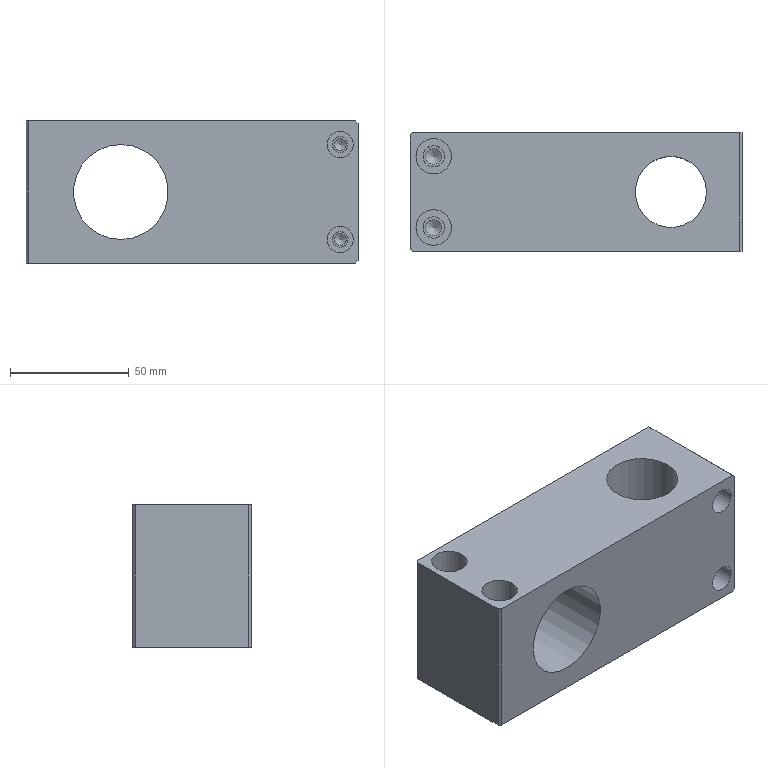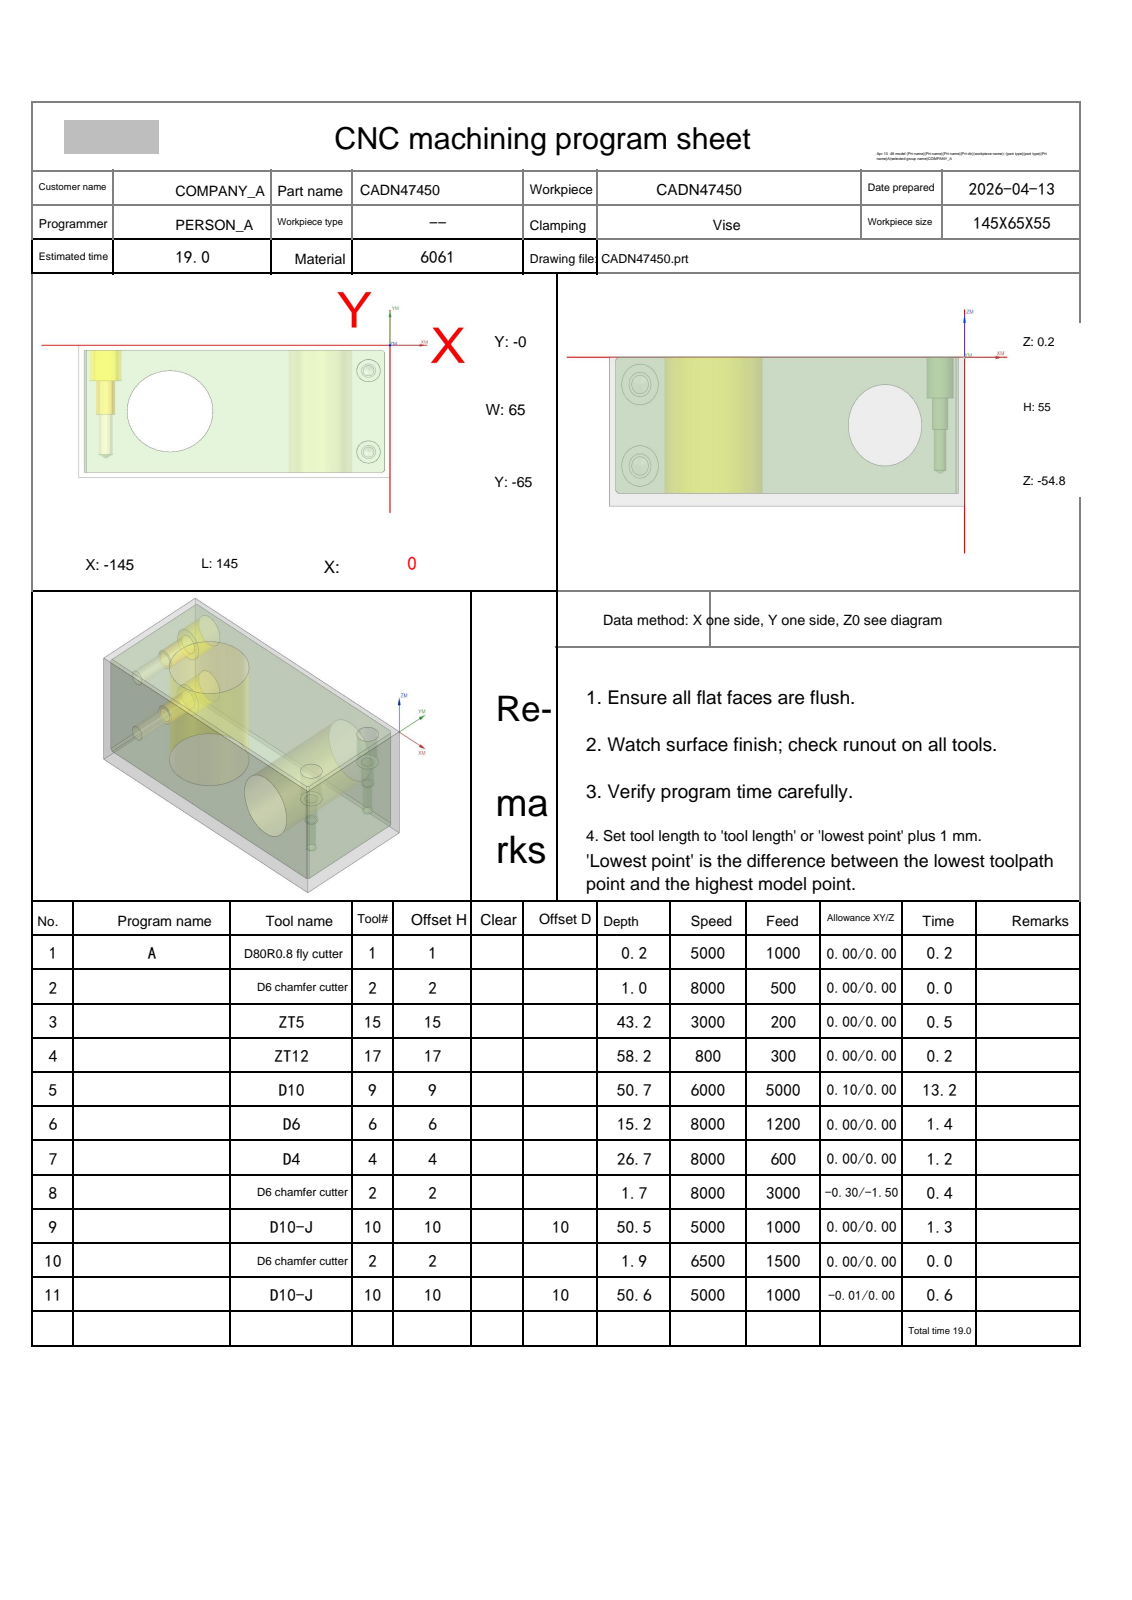NC program | NX | posted by the shop | part box 140 x 50 x 60 mm
Lines 4207 to 4750 of 4750:
N6 T06 M06
(D6  D=6. R=0. H=06 ce=0.00 di=0.00)
G00 G90 G54 X-10. Y-52.5 M03 S8000
G43 H06 Z20.
M08
Z.5
G03 X-8.75 Y-53.75 I1.25 J0.0 F1200.
X-7.5 Y-52.5 I0.0 J1.25
X-7.5 Y-52.5 Z.2 I-2.5 J0.0
X-7.5 Y-52.5 Z-.1 I-2.5 J0.0
X-7.5 Y-52.5 Z-.4 I-2.5 J0.0
X-7.5 Y-52.5 Z-.7 I-2.5 J0.0
X-7.5 Y-52.5 Z-1. I-2.5 J0.0
X-7.5 Y-52.5 Z-1.3 I-2.5 J0.0
X-7.5 Y-52.5 Z-1.6 I-2.5 J0.0
X-7.5 Y-52.5 Z-1.9 I-2.5 J0.0
X-7.5 Y-52.5 Z-2.2 I-2.5 J0.0
X-7.5 Y-52.5 Z-2.5 I-2.5 J0.0
X-7.5 Y-52.5 Z-2.8 I-2.5 J0.0
X-7.5 Y-52.5 Z-3.1 I-2.5 J0.0
X-7.5 Y-52.5 Z-3.4 I-2.5 J0.0
X-7.5 Y-52.5 Z-3.7 I-2.5 J0.0
X-7.5 Y-52.5 Z-4. I-2.5 J0.0
X-7.5 Y-52.5 Z-4.3 I-2.5 J0.0
X-7.5 Y-52.5 Z-4.6 I-2.5 J0.0
X-7.5 Y-52.5 Z-4.9 I-2.5 J0.0
X-7.5 Y-52.5 Z-5.2 I-2.5 J0.0
X-7.5 Y-52.5 Z-5.5 I-2.5 J0.0
X-7.5 Y-52.5 Z-5.8 I-2.5 J0.0
X-7.5 Y-52.5 Z-6.1 I-2.5 J0.0
X-7.5 Y-52.5 Z-6.4 I-2.5 J0.0
X-7.5 Y-52.5 Z-6.7 I-2.5 J0.0
X-7.5 Y-52.5 Z-7. I-2.5 J0.0
X-7.5 Y-52.5 Z-7.3 I-2.5 J0.0
X-7.5 Y-52.5 Z-7.6 I-2.5 J0.0
X-7.5 Y-52.5 Z-7.9 I-2.5 J0.0
X-7.5 Y-52.5 Z-8.2 I-2.5 J0.0
X-7.5 Y-52.5 Z-8.5 I-2.5 J0.0
X-7.5 Y-52.5 Z-8.8 I-2.5 J0.0
X-7.5 Y-52.5 Z-9.1 I-2.5 J0.0
X-7.5 Y-52.5 Z-9.4 I-2.5 J0.0
X-7.5 Y-52.5 Z-9.7 I-2.5 J0.0
X-7.5 Y-52.5 Z-10. I-2.5 J0.0
X-7.5 Y-52.5 Z-10.3 I-2.5 J0.0
X-7.5 Y-52.5 Z-10.6 I-2.5 J0.0
X-7.5 Y-52.5 Z-10.9 I-2.5 J0.0
X-7.5 Y-52.5 Z-11.2 I-2.5 J0.0
X-7.5 Y-52.5 Z-11.5 I-2.5 J0.0
X-7.5 Y-52.5 Z-11.8 I-2.5 J0.0
X-7.5 Y-52.5 Z-12.1 I-2.5 J0.0
X-7.5 Y-52.5 Z-12.4 I-2.5 J0.0
X-7.5 Y-52.5 Z-12.7 I-2.5 J0.0
X-7.5 Y-52.5 Z-13. I-2.5 J0.0
X-7.5 Y-52.5 Z-13.3 I-2.5 J0.0
X-7.5 Y-52.5 Z-13.6 I-2.5 J0.0
X-7.5 Y-52.5 Z-13.9 I-2.5 J0.0
X-7.5 Y-52.5 Z-14.2 I-2.5 J0.0
X-7.5 Y-52.5 Z-14.5 I-2.5 J0.0
X-7.5 Y-52.5 Z-14.8 I-2.5 J0.0
X-11.25 Y-54.665 Z-15. I-2.5 J0.0
X-10. Y-55. I1.25 J2.165
X-7.5 Y-52.5 I0.0 J2.5
X-10. Y-50. I-2.5 J0.0
X-12.5 Y-52.5 I0.0 J-2.5
X-11.25 Y-54.665 I2.5 J0.0
X-10.625 Y-54.833 I.625 J1.083
X-9.375 Y-53.583 I0.0 J1.25
X-10. Y-52.5 I-1.25 J0.0
G00 Z20.
Y-12.5
Z.5
G03 X-8.75 Y-13.75 I1.25 J0.0
X-7.5 Y-12.5 I0.0 J1.25
X-7.5 Y-12.5 Z.2 I-2.5 J0.0
X-7.5 Y-12.5 Z-.1 I-2.5 J0.0
X-7.5 Y-12.5 Z-.4 I-2.5 J0.0
X-7.5 Y-12.5 Z-.7 I-2.5 J0.0
X-7.5 Y-12.5 Z-1. I-2.5 J0.0
X-7.5 Y-12.5 Z-1.3 I-2.5 J0.0
X-7.5 Y-12.5 Z-1.6 I-2.5 J0.0
X-7.5 Y-12.5 Z-1.9 I-2.5 J0.0
X-7.5 Y-12.5 Z-2.2 I-2.5 J0.0
X-7.5 Y-12.5 Z-2.5 I-2.5 J0.0
X-7.5 Y-12.5 Z-2.8 I-2.5 J0.0
X-7.5 Y-12.5 Z-3.1 I-2.5 J0.0
X-7.5 Y-12.5 Z-3.4 I-2.5 J0.0
X-7.5 Y-12.5 Z-3.7 I-2.5 J0.0
X-7.5 Y-12.5 Z-4. I-2.5 J0.0
X-7.5 Y-12.5 Z-4.3 I-2.5 J0.0
X-7.5 Y-12.5 Z-4.6 I-2.5 J0.0
X-7.5 Y-12.5 Z-4.9 I-2.5 J0.0
X-7.5 Y-12.5 Z-5.2 I-2.5 J0.0
X-7.5 Y-12.5 Z-5.5 I-2.5 J0.0
X-7.5 Y-12.5 Z-5.8 I-2.5 J0.0
X-7.5 Y-12.5 Z-6.1 I-2.5 J0.0
X-7.5 Y-12.5 Z-6.4 I-2.5 J0.0
X-7.5 Y-12.5 Z-6.7 I-2.5 J0.0
X-7.5 Y-12.5 Z-7. I-2.5 J0.0
X-7.5 Y-12.5 Z-7.3 I-2.5 J0.0
X-7.5 Y-12.5 Z-7.6 I-2.5 J0.0
X-7.5 Y-12.5 Z-7.9 I-2.5 J0.0
X-7.5 Y-12.5 Z-8.2 I-2.5 J0.0
X-7.5 Y-12.5 Z-8.5 I-2.5 J0.0
X-7.5 Y-12.5 Z-8.8 I-2.5 J0.0
X-7.5 Y-12.5 Z-9.1 I-2.5 J0.0
X-7.5 Y-12.5 Z-9.4 I-2.5 J0.0
X-7.5 Y-12.5 Z-9.7 I-2.5 J0.0
X-7.5 Y-12.5 Z-10. I-2.5 J0.0
X-7.5 Y-12.5 Z-10.3 I-2.5 J0.0
X-7.5 Y-12.5 Z-10.6 I-2.5 J0.0
X-7.5 Y-12.5 Z-10.9 I-2.5 J0.0
X-7.5 Y-12.5 Z-11.2 I-2.5 J0.0
X-7.5 Y-12.5 Z-11.5 I-2.5 J0.0
X-7.5 Y-12.5 Z-11.8 I-2.5 J0.0
X-7.5 Y-12.5 Z-12.1 I-2.5 J0.0
X-7.5 Y-12.5 Z-12.4 I-2.5 J0.0
X-7.5 Y-12.5 Z-12.7 I-2.5 J0.0
X-7.5 Y-12.5 Z-13. I-2.5 J0.0
X-7.5 Y-12.5 Z-13.3 I-2.5 J0.0
X-7.5 Y-12.5 Z-13.6 I-2.5 J0.0
X-7.5 Y-12.5 Z-13.9 I-2.5 J0.0
X-7.5 Y-12.5 Z-14.2 I-2.5 J0.0
X-7.5 Y-12.5 Z-14.5 I-2.5 J0.0
X-7.5 Y-12.5 Z-14.8 I-2.5 J0.0
X-11.25 Y-14.665 Z-15. I-2.5 J0.0
X-10. Y-15. I1.25 J2.165
X-7.5 Y-12.5 I0.0 J2.5
X-10. Y-10. I-2.5 J0.0
X-12.5 Y-12.5 I0.0 J-2.5
X-11.25 Y-14.665 I2.5 J0.0
X-10.625 Y-14.833 I.625 J1.083
X-9.375 Y-13.583 I0.0 J1.25
X-10. Y-12.5 I-1.25 J0.0
G00 Z20.
G91 G28 Z0.0
M05
M09
G91 G28 Z0.0
M01
N7 T04 M06
(D4  D=4. R=0. H=04 ce=0.00 di=0.00)
G00 G90 G54 X-10. Y-52.5 M03 S8000
G43 H04 Z20.
M08
Z-14.5
G03 X-9.35 Y-53.15 I.65 J0.0 F600.
X-8.7 Y-52.5 I0.0 J.65
X-8.7 Y-52.5 Z-14.8 I-1.3 J0.0
X-8.7 Y-52.5 Z-15.1 I-1.3 J0.0
X-8.7 Y-52.5 Z-15.4 I-1.3 J0.0
X-8.7 Y-52.5 Z-15.7 I-1.3 J0.0
X-8.7 Y-52.5 Z-16. I-1.3 J0.0
X-8.7 Y-52.5 Z-16.3 I-1.3 J0.0
X-8.7 Y-52.5 Z-16.6 I-1.3 J0.0
X-8.7 Y-52.5 Z-16.9 I-1.3 J0.0
X-8.7 Y-52.5 Z-17.2 I-1.3 J0.0
X-8.7 Y-52.5 Z-17.5 I-1.3 J0.0
X-8.7 Y-52.5 Z-17.8 I-1.3 J0.0
X-8.7 Y-52.5 Z-18.1 I-1.3 J0.0
X-8.7 Y-52.5 Z-18.4 I-1.3 J0.0
X-8.7 Y-52.5 Z-18.7 I-1.3 J0.0
X-8.7 Y-52.5 Z-19. I-1.3 J0.0
X-8.7 Y-52.5 Z-19.3 I-1.3 J0.0
X-8.7 Y-52.5 Z-19.6 I-1.3 J0.0
X-8.7 Y-52.5 Z-19.9 I-1.3 J0.0
X-8.7 Y-52.5 Z-20.2 I-1.3 J0.0
X-8.7 Y-52.5 Z-20.5 I-1.3 J0.0
X-8.7 Y-52.5 Z-20.8 I-1.3 J0.0
X-8.7 Y-52.5 Z-21.1 I-1.3 J0.0
X-8.7 Y-52.5 Z-21.4 I-1.3 J0.0
X-8.7 Y-52.5 Z-21.7 I-1.3 J0.0
X-8.7 Y-52.5 Z-22. I-1.3 J0.0
X-8.7 Y-52.5 Z-22.3 I-1.3 J0.0
X-8.7 Y-52.5 Z-22.6 I-1.3 J0.0
X-8.7 Y-52.5 Z-22.9 I-1.3 J0.0
X-8.7 Y-52.5 Z-23.2 I-1.3 J0.0
X-8.7 Y-52.5 Z-23.5 I-1.3 J0.0
X-8.7 Y-52.5 Z-23.8 I-1.3 J0.0
X-8.7 Y-52.5 Z-24.1 I-1.3 J0.0
X-8.7 Y-52.5 Z-24.4 I-1.3 J0.0
X-8.7 Y-52.5 Z-24.7 I-1.3 J0.0
X-8.7 Y-52.5 Z-25. I-1.3 J0.0
X-8.7 Y-52.5 Z-25.3 I-1.3 J0.0
X-8.7 Y-52.5 Z-25.6 I-1.3 J0.0
X-8.7 Y-52.5 Z-25.9 I-1.3 J0.0
X-8.7 Y-52.5 Z-26.2 I-1.3 J0.0
X-8.7 Y-52.5 Z-26.5 I-1.3 J0.0
X-10. Y-51.2 I-1.3 J0.0
X-11.3 Y-52.5 I0.0 J-1.3
X-10. Y-53.8 I1.3 J0.0
X-8.7 Y-52.5 I0.0 J1.3
X-9.35 Y-51.85 I-.65 J0.0
X-10. Y-52.5 I0.0 J-.65
G00 Z20.
Y-12.5
Z-14.5
G03 X-9.35 Y-13.15 I.65 J0.0
X-8.7 Y-12.5 I0.0 J.65
X-8.7 Y-12.5 Z-14.8 I-1.3 J0.0
X-8.7 Y-12.5 Z-15.1 I-1.3 J0.0
X-8.7 Y-12.5 Z-15.4 I-1.3 J0.0
X-8.7 Y-12.5 Z-15.7 I-1.3 J0.0
X-8.7 Y-12.5 Z-16. I-1.3 J0.0
X-8.7 Y-12.5 Z-16.3 I-1.3 J0.0
X-8.7 Y-12.5 Z-16.6 I-1.3 J0.0
X-8.7 Y-12.5 Z-16.9 I-1.3 J0.0
X-8.7 Y-12.5 Z-17.2 I-1.3 J0.0
X-8.7 Y-12.5 Z-17.5 I-1.3 J0.0
X-8.7 Y-12.5 Z-17.8 I-1.3 J0.0
X-8.7 Y-12.5 Z-18.1 I-1.3 J0.0
X-8.7 Y-12.5 Z-18.4 I-1.3 J0.0
X-8.7 Y-12.5 Z-18.7 I-1.3 J0.0
X-8.7 Y-12.5 Z-19. I-1.3 J0.0
X-8.7 Y-12.5 Z-19.3 I-1.3 J0.0
X-8.7 Y-12.5 Z-19.6 I-1.3 J0.0
X-8.7 Y-12.5 Z-19.9 I-1.3 J0.0
X-8.7 Y-12.5 Z-20.2 I-1.3 J0.0
X-8.7 Y-12.5 Z-20.5 I-1.3 J0.0
X-8.7 Y-12.5 Z-20.8 I-1.3 J0.0
X-8.7 Y-12.5 Z-21.1 I-1.3 J0.0
X-8.7 Y-12.5 Z-21.4 I-1.3 J0.0
X-8.7 Y-12.5 Z-21.7 I-1.3 J0.0
X-8.7 Y-12.5 Z-22. I-1.3 J0.0
X-8.7 Y-12.5 Z-22.3 I-1.3 J0.0
X-8.7 Y-12.5 Z-22.6 I-1.3 J0.0
X-8.7 Y-12.5 Z-22.9 I-1.3 J0.0
X-8.7 Y-12.5 Z-23.2 I-1.3 J0.0
X-8.7 Y-12.5 Z-23.5 I-1.3 J0.0
X-8.7 Y-12.5 Z-23.8 I-1.3 J0.0
X-8.7 Y-12.5 Z-24.1 I-1.3 J0.0
X-8.7 Y-12.5 Z-24.4 I-1.3 J0.0
X-8.7 Y-12.5 Z-24.7 I-1.3 J0.0
X-8.7 Y-12.5 Z-25. I-1.3 J0.0
X-8.7 Y-12.5 Z-25.3 I-1.3 J0.0
X-8.7 Y-12.5 Z-25.6 I-1.3 J0.0
X-8.7 Y-12.5 Z-25.9 I-1.3 J0.0
X-8.7 Y-12.5 Z-26.2 I-1.3 J0.0
X-8.7 Y-12.5 Z-26.5 I-1.3 J0.0
X-10. Y-11.2 I-1.3 J0.0
X-11.3 Y-12.5 I0.0 J-1.3
X-10. Y-13.8 I1.3 J0.0
X-8.7 Y-12.5 I0.0 J1.3
X-9.35 Y-11.85 I-.65 J0.0
X-10. Y-12.5 I0.0 J-.65
G00 Z20.
G91 G28 Z0.0
M05
M09
G91 G28 Z0.0
M01
N8 T02 M06
(D6 chamfer cutter  D=6. R=0. H=02 ce=0.00 di=0.00)
G00 G90 G54 X-141.961 Y-1.293 M03 S8000
G43 H02 Z20.
M08
Z2.935
G01 Z-1.5 F3000.
X-141.789 Y-1.233
X-141.5 Y-1.2
X-72.5
X-3.5
X-3.246 Y-1.225
X-3.003 Y-1.299
X-2.778 Y-1.419
X-2.581 Y-1.581
X-1.581 Y-2.581
X-1.419 Y-2.778
X-1.299 Y-3.003
X-1.225 Y-3.246
X-1.2 Y-3.5
Y-61.5
X-1.225 Y-61.754
X-1.299 Y-61.997
X-1.419 Y-62.222
X-1.581 Y-62.419
X-2.581 Y-63.419
X-2.778 Y-63.581
X-3.003 Y-63.701
X-3.246 Y-63.775
X-3.5 Y-63.8
X-141.5
X-141.789 Y-63.767
X-141.961 Y-63.707
Z2.935
G00 Z20.
X-102.225 Y-14.62
Z2.117
G01 Z-1.5
G03 X-102.154 Y-14.336 I-.529 J.284
X-102.47 Y-13.807 I-.6 J0.0
G01 X-102.5 Y-13.8
G03 X-121.2 Y-32.5 I0.0 J-18.7
X-102.5 Y-51.2 I18.7 J0.0
X-83.8 Y-32.5 I0.0 J18.7
X-102.5 Y-13.8 I-18.7 J0.0
G01 X-102.53 Y-13.807
G03 X-102.846 Y-14.336 I.284 J-.529
X-102.775 Y-14.62 I.6 J0.0
G01 Z2.117
G00 Z20.
G00 G90 X-13. Y-54.1 M03 S8000
Z20.
Z-.7
G01 Z-1.2 F800.
G03 X-10. Y-57.1 I3. J0.0
X-5.4 Y-52.5 I0.0 J4.6
X-10. Y-47.9 I-4.6 J0.0
X-14.6 Y-52.5 I0.0 J-4.6
X-10. Y-57.1 I4.6 J0.0
X-7. Y-54.1 I0.0 J3.
G01 Z-.7
G00 Z20.
X-13. Y-14.1
Z-.7
G01 Z-1.2
G03 X-10. Y-17.1 I3. J0.0
X-5.4 Y-12.5 I0.0 J4.6
X-10. Y-7.9 I-4.6 J0.0
X-14.6 Y-12.5 I0.0 J-4.6
X-10. Y-17.1 I4.6 J0.0
X-7. Y-14.1 I0.0 J3.
G01 Z-.7
G00 Z20.
G00 G90 X-99.5 Y-16.7 M03 S8000
Z20.
Z-1.
G01 Z-1.5 F1000.
G03 X-102.5 Y-13.7 I-3. J0.0
X-121.3 Y-32.5 I0.0 J-18.8
X-102.5 Y-51.3 I18.8 J0.0
X-83.7 Y-32.5 I0.0 J18.8
X-102.5 Y-13.7 I-18.8 J0.0
X-105.5 Y-16.7 I0.0 J-3.
G01 Z-1.
G00 Z20.
G91 G28 Z0.0
M05
M09
G91 G28 Z0.0
M01
N9 T10 M06
(D10-J  D=10. R=0. H=10 ce=0.00 di=0.00)
G00 G90 G54 X-143.513 Y3.616 M03 S5000
G43 H10 Z20.
M08
Z-16.267
G01 Z-16.767 F1000.
G41 D10
X-143.497 Y3.417
G03 X-142.5 Y2.5 I.997 J.083
G01 X-3.5
G02 X.036 Y1.036 I0.0 J-5.
G01 X1.036 Y.036
G02 X2.5 Y-3.5 I-3.536 J-3.536
G01 Y-61.5
G02 X1.036 Y-65.036 I-5. J0.0
G01 X.036 Y-66.036
G02 X-3.5 Y-67.5 I-3.536 J3.536
G01 X-142.5
G02 X-147.5 Y-62.5 I0.0 J5.
G01 Y-2.5
G02 X-142.5 Y2.5 I5. J0.0
G01 X-142.
G03 X-141. Y3.5 I0.0 J1.
G01 G40 Y3.7
Z-16.267
G00 Z20.
X-143.513 Y3.616
Z-33.033
G01 Z-33.533
G41 D10
X-143.497 Y3.417
G03 X-142.5 Y2.5 I.997 J.083
G01 X-3.5
G02 X.036 Y1.036 I0.0 J-5.
G01 X1.036 Y.036
G02 X2.5 Y-3.5 I-3.536 J-3.536
G01 Y-61.5
G02 X1.036 Y-65.036 I-5. J0.0
G01 X.036 Y-66.036
G02 X-3.5 Y-67.5 I-3.536 J3.536
G01 X-142.5
G02 X-147.5 Y-62.5 I0.0 J5.
G01 Y-2.5
G02 X-142.5 Y2.5 I5. J0.0
G01 X-142.
G03 X-141. Y3.5 I0.0 J1.
G01 G40 Y3.7
Z-33.033
G00 Z20.
X-143.513 Y3.616
Z-49.8
G01 Z-50.3
G41 D10
X-143.497 Y3.417
G03 X-142.5 Y2.5 I.997 J.083
G01 X-3.5
G02 X.036 Y1.036 I0.0 J-5.
G01 X1.036 Y.036
G02 X2.5 Y-3.5 I-3.536 J-3.536
G01 Y-61.5
G02 X1.036 Y-65.036 I-5. J0.0
G01 X.036 Y-66.036
G02 X-3.5 Y-67.5 I-3.536 J3.536
G01 X-142.5
G02 X-147.5 Y-62.5 I0.0 J5.
G01 Y-2.5
G02 X-142.5 Y2.5 I5. J0.0
G01 X-142.
G03 X-141. Y3.5 I0.0 J1.
G01 G40 Y3.7
Z-49.8
G00 Z20.
G91 G28 Z0.0
M05
M09
G91 G28 Z0.0
M01
N10 T02 M06
(D6 chamfer cutter  D=6. R=0. H=02 ce=0.00 di=0.00)
G00 G90 G54 X-143.208 Y-65.4 M03 S6500
G43 H02 Z20.
M08
Z-.2
G01 Z-1.7 F1500.
X-143.199 Y-65.332
X-143.2 Y-65.263
Y.263
X-143.199 Y.332
X-143.208 Y.4
Z-.2
G00 Z20.
G91 G28 Z0.0
M05
M09
G91 G28 Z0.0
M01
N11 T10 M06
(D10-J  D=10. R=0. H=10 ce=-0.01 di=0.00)
G00 G90 G54 X-104. Y-45.726 M03 S5000
G43 H10 Z10.2
M08
Z-6.9
G01 Z-8.4 F1000.
G41 D10
Y-46.01
G03 X-102.5 Y-47.51 I1.5 J0.0
X-87.49 Y-32.5 I0.0 J15.01
X-102.5 Y-17.49 I-15.01 J0.0
X-117.51 Y-32.5 I0.0 J-15.01
X-102.5 Y-47.51 I15.01 J0.0
X-102.1 Y-47.505 I0.0 J15.01
X-100.64 Y-46.005 I-.04 J1.499
G01 X-100.641 Y-45.965
X-100.643 Y-45.882
G40 X-100.648 Y-45.682
Z-6.9
G00 X-104. Y-45.726
Z-15.3
G01 Z-16.8
G41 D10
Y-46.01
G03 X-102.5 Y-47.51 I1.5 J0.0
X-87.49 Y-32.5 I0.0 J15.01
X-102.5 Y-17.49 I-15.01 J0.0
X-117.51 Y-32.5 I0.0 J-15.01
X-102.5 Y-47.51 I15.01 J0.0
X-102.1 Y-47.505 I0.0 J15.01
X-100.64 Y-46.005 I-.04 J1.499
G01 X-100.641 Y-45.965
X-100.643 Y-45.882
G40 X-100.648 Y-45.682
Z-15.3
G00 X-104. Y-45.726
Z-23.7
G01 Z-25.2
G41 D10
Y-46.01
G03 X-102.5 Y-47.51 I1.5 J0.0
X-87.49 Y-32.5 I0.0 J15.01
X-102.5 Y-17.49 I-15.01 J0.0
X-117.51 Y-32.5 I0.0 J-15.01
X-102.5 Y-47.51 I15.01 J0.0
X-102.1 Y-47.505 I0.0 J15.01
X-100.64 Y-46.005 I-.04 J1.499
G01 X-100.641 Y-45.965
X-100.643 Y-45.882
G40 X-100.648 Y-45.682
Z-23.7
G00 X-104. Y-45.726
Z-32.1
G01 Z-33.6
G41 D10
Y-46.01
G03 X-102.5 Y-47.51 I1.5 J0.0
X-87.49 Y-32.5 I0.0 J15.01
X-102.5 Y-17.49 I-15.01 J0.0
X-117.51 Y-32.5 I0.0 J-15.01
X-102.5 Y-47.51 I15.01 J0.0
X-102.1 Y-47.505 I0.0 J15.01
X-100.64 Y-46.005 I-.04 J1.499
G01 X-100.641 Y-45.965
X-100.643 Y-45.882
G40 X-100.648 Y-45.682
Z-32.1
G00 X-104. Y-45.726
Z-40.5
G01 Z-42.
G41 D10
Y-46.01
G03 X-102.5 Y-47.51 I1.5 J0.0
X-87.49 Y-32.5 I0.0 J15.01
X-102.5 Y-17.49 I-15.01 J0.0
X-117.51 Y-32.5 I0.0 J-15.01
X-102.5 Y-47.51 I15.01 J0.0
X-102.1 Y-47.505 I0.0 J15.01
X-100.64 Y-46.005 I-.04 J1.499
G01 X-100.641 Y-45.965
X-100.643 Y-45.882
G40 X-100.648 Y-45.682
Z-40.5
G00 X-104. Y-45.726
Z-48.9
G01 Z-50.4
G41 D10
Y-46.01
G03 X-102.5 Y-47.51 I1.5 J0.0
X-87.49 Y-32.5 I0.0 J15.01
X-102.5 Y-17.49 I-15.01 J0.0
X-117.51 Y-32.5 I0.0 J-15.01
X-102.5 Y-47.51 I15.01 J0.0
X-102.1 Y-47.505 I0.0 J15.01
X-100.64 Y-46.005 I-.04 J1.499
G01 X-100.641 Y-45.965
X-100.643 Y-45.882
G40 X-100.648 Y-45.682
Z-48.9
G00 Z10.2
M05
M09
G91 G28 Z0.0
G91 G28 Y0.0
M30
%